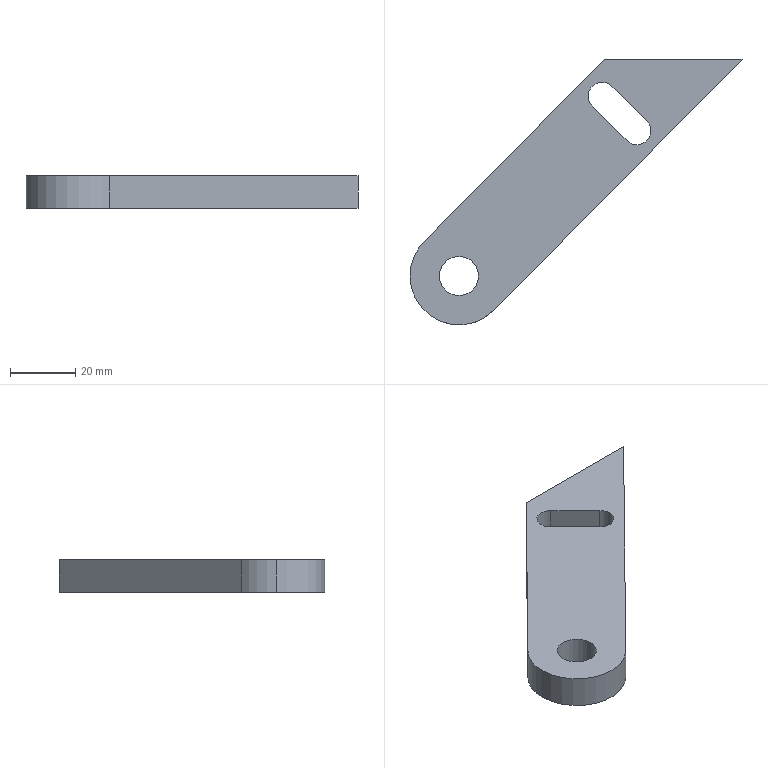Part | STEP file | Tensioning pulley fixing plate SGN-2-19 | 1 solid | 14 faces | box 101.738 x 81.439 x 10 mm | volume 28553 mm3 | cylinder 7 | plane 7 | commonest cylinder face diameters 8.6 x3 12 x2 30 x2
STEP:
#1=CARTESIAN_POINT('',(0.,0.,0.));
#2=DIRECTION('',(0.,0.,1.));
#3=DIRECTION('',(1.,0.,0.));
#4=AXIS2_PLACEMENT_3D('',#1,#2,#3);
#5=CARTESIAN_POINT('',(12.996,-18.86,0.));
#6=VERTEX_POINT('',#5);
#7=CARTESIAN_POINT('',(12.996,-18.86,10.));
#8=VERTEX_POINT('',#7);
#9=CARTESIAN_POINT('',(12.996,-18.86,0.));
#10=DIRECTION('',(0.,0.,1.));
#11=VECTOR('',#10,1.);
#12=LINE('',#9,#11);
#13=CARTESIAN_POINT('',(9.973,-21.919,0.));
#14=DIRECTION('',(0.,0.,1.));
#15=DIRECTION('',(1.,0.,0.));
#16=AXIS2_PLACEMENT_3D('',#13,#14,#15);
#17=CYLINDRICAL_SURFACE('',#16,4.3);
#18=CARTESIAN_POINT('',(0.7914,0.));
#19=DIRECTION('',(0.,1.));
#20=VECTOR('',#19,1.);
#21=LINE('',#18,#20);
#22=(GEOMETRIC_REPRESENTATION_CONTEXT(2)PARAMETRIC_REPRESENTATION_CONTEXT()REPRESENTATION_CONTEXT('',''));
#23=DEFINITIONAL_REPRESENTATION('',(#21),#22);
#24=PCURVE('',#17,#23);
#25=CARTESIAN_POINT('',(2.326,-8.317,0.));
#26=DIRECTION('',(0.7029,0.7113,0.));
#27=DIRECTION('',(-0.7113,0.7029,0.));
#28=AXIS2_PLACEMENT_3D('',#25,#26,#27);
#29=PLANE('',#28);
#30=CARTESIAN_POINT('',(-15.,0.));
#31=DIRECTION('',(0.,1.));
#32=VECTOR('',#31,1.);
#33=LINE('',#30,#32);
#34=(GEOMETRIC_REPRESENTATION_CONTEXT(2)PARAMETRIC_REPRESENTATION_CONTEXT()REPRESENTATION_CONTEXT('',''));
#35=DEFINITIONAL_REPRESENTATION('',(#33),#34);
#36=PCURVE('',#29,#35);
#37=SURFACE_CURVE('',#12,(#24,#36),.PCURVE_S1.);
#38=EDGE_CURVE('',#6,#8,#37,.T.);
#39=ORIENTED_EDGE('',*,*,#38,.T.);
#40=CARTESIAN_POINT('',(14.273,-21.919,10.));
#41=VERTEX_POINT('',#40);
#42=CARTESIAN_POINT('',(9.973,-21.919,10.));
#43=DIRECTION('',(0.,0.,1.));
#44=DIRECTION('',(1.,0.,0.));
#45=AXIS2_PLACEMENT_3D('',#42,#43,#44);
#46=CIRCLE('',#45,4.3);
#47=CARTESIAN_POINT('',(0.,10.));
#48=DIRECTION('',(1.,0.));
#49=VECTOR('',#48,1.);
#50=LINE('',#47,#49);
#51=(GEOMETRIC_REPRESENTATION_CONTEXT(2)PARAMETRIC_REPRESENTATION_CONTEXT()REPRESENTATION_CONTEXT('',''));
#52=DEFINITIONAL_REPRESENTATION('',(#50),#51);
#53=PCURVE('',#17,#52);
#54=CARTESIAN_POINT('',(-44.563,-66.439,10.));
#55=DIRECTION('',(0.,0.,1.));
#56=DIRECTION('',(1.,0.,0.));
#57=AXIS2_PLACEMENT_3D('',#54,#55,#56);
#58=PLANE('',#57);
#59=CARTESIAN_POINT('',(54.536,44.521));
#60=DIRECTION('',(1.,0.));
#61=AXIS2_PLACEMENT_2D('',#59,#60);
#62=CIRCLE('',#61,4.3);
#63=(GEOMETRIC_REPRESENTATION_CONTEXT(2)PARAMETRIC_REPRESENTATION_CONTEXT()REPRESENTATION_CONTEXT('',''));
#64=DEFINITIONAL_REPRESENTATION('',(#62),#63);
#65=PCURVE('',#58,#64);
#66=SURFACE_CURVE('',#46,(#53,#65),.PCURVE_S1.);
#67=EDGE_CURVE('',#41,#8,#66,.T.);
#68=ORIENTED_EDGE('',*,*,#67,.F.);
#69=CARTESIAN_POINT('',(14.273,-21.919,0.));
#70=VERTEX_POINT('',#69);
#71=CARTESIAN_POINT('',(14.273,-21.919,0.));
#72=DIRECTION('',(0.,0.,1.));
#73=VECTOR('',#72,1.);
#74=LINE('',#71,#73);
#75=CARTESIAN_POINT('',(0.,0.));
#76=DIRECTION('',(0.,1.));
#77=VECTOR('',#76,1.);
#78=LINE('',#75,#77);
#79=(GEOMETRIC_REPRESENTATION_CONTEXT(2)PARAMETRIC_REPRESENTATION_CONTEXT()REPRESENTATION_CONTEXT('',''));
#80=DEFINITIONAL_REPRESENTATION('',(#78),#79);
#81=PCURVE('',#17,#80);
#82=CARTESIAN_POINT('',(9.973,-21.919,0.));
#83=DIRECTION('',(0.,0.,1.));
#84=DIRECTION('',(1.,0.,0.));
#85=AXIS2_PLACEMENT_3D('',#82,#83,#84);
#86=CYLINDRICAL_SURFACE('',#85,4.3);
#87=CARTESIAN_POINT('',(6.283,0.));
#88=DIRECTION('',(0.,1.));
#89=VECTOR('',#88,1.);
#90=LINE('',#87,#89);
#91=(GEOMETRIC_REPRESENTATION_CONTEXT(2)PARAMETRIC_REPRESENTATION_CONTEXT()REPRESENTATION_CONTEXT('',''));
#92=DEFINITIONAL_REPRESENTATION('',(#90),#91);
#93=PCURVE('',#86,#92);
#94=SURFACE_CURVE('',#74,(#81,#93),.PCURVE_S1.);
#95=EDGE_CURVE('',#70,#41,#94,.T.);
#96=ORIENTED_EDGE('',*,*,#95,.F.);
#97=CARTESIAN_POINT('',(9.973,-21.919,0.));
#98=DIRECTION('',(0.,0.,1.));
#99=DIRECTION('',(1.,0.,0.));
#100=AXIS2_PLACEMENT_3D('',#97,#98,#99);
#101=CIRCLE('',#100,4.3);
#102=CARTESIAN_POINT('',(0.,0.));
#103=DIRECTION('',(1.,0.));
#104=VECTOR('',#103,1.);
#105=LINE('',#102,#104);
#106=(GEOMETRIC_REPRESENTATION_CONTEXT(2)PARAMETRIC_REPRESENTATION_CONTEXT()REPRESENTATION_CONTEXT('',''));
#107=DEFINITIONAL_REPRESENTATION('',(#105),#106);
#108=PCURVE('',#17,#107);
#109=CARTESIAN_POINT('',(-44.563,-66.439,0.));
#110=DIRECTION('',(0.,0.,1.));
#111=DIRECTION('',(1.,0.,0.));
#112=AXIS2_PLACEMENT_3D('',#109,#110,#111);
#113=PLANE('',#112);
#114=CARTESIAN_POINT('',(54.536,44.521));
#115=DIRECTION('',(1.,0.));
#116=AXIS2_PLACEMENT_2D('',#114,#115);
#117=CIRCLE('',#116,4.3);
#118=(GEOMETRIC_REPRESENTATION_CONTEXT(2)PARAMETRIC_REPRESENTATION_CONTEXT()REPRESENTATION_CONTEXT('',''));
#119=DEFINITIONAL_REPRESENTATION('',(#117),#118);
#120=PCURVE('',#113,#119);
#121=SURFACE_CURVE('',#101,(#108,#120),.PCURVE_S1.);
#122=EDGE_CURVE('',#70,#6,#121,.T.);
#123=ORIENTED_EDGE('',*,*,#122,.T.);
#124=EDGE_LOOP('',(#39,#68,#96,#123));
#125=FACE_BOUND('',#124,.F.);
#126=ADVANCED_FACE('',(#125),#17,.F.);
#127=CARTESIAN_POINT('',(-38.563,-66.439,0.));
#128=VERTEX_POINT('',#127);
#129=CARTESIAN_POINT('',(-38.563,-66.439,10.));
#130=VERTEX_POINT('',#129);
#131=CARTESIAN_POINT('',(-38.563,-66.439,10.));
#132=DIRECTION('',(0.,0.,1.));
#133=VECTOR('',#132,1.);
#134=LINE('',#131,#133);
#135=CARTESIAN_POINT('',(-44.563,-66.439,10.));
#136=DIRECTION('',(0.,0.,1.));
#137=DIRECTION('',(1.,0.,0.));
#138=AXIS2_PLACEMENT_3D('',#135,#136,#137);
#139=CYLINDRICAL_SURFACE('',#138,6.);
#140=CARTESIAN_POINT('',(6.283,0.));
#141=DIRECTION('',(0.,1.));
#142=VECTOR('',#141,1.);
#143=LINE('',#140,#142);
#144=(GEOMETRIC_REPRESENTATION_CONTEXT(2)PARAMETRIC_REPRESENTATION_CONTEXT()REPRESENTATION_CONTEXT('',''));
#145=DEFINITIONAL_REPRESENTATION('',(#143),#144);
#146=PCURVE('',#139,#145);
#147=CARTESIAN_POINT('',(-44.563,-66.439,10.));
#148=DIRECTION('',(0.,0.,1.));
#149=DIRECTION('',(1.,0.,0.));
#150=AXIS2_PLACEMENT_3D('',#147,#148,#149);
#151=CYLINDRICAL_SURFACE('',#150,6.);
#152=CARTESIAN_POINT('',(0.,0.));
#153=DIRECTION('',(0.,1.));
#154=VECTOR('',#153,1.);
#155=LINE('',#152,#154);
#156=(GEOMETRIC_REPRESENTATION_CONTEXT(2)PARAMETRIC_REPRESENTATION_CONTEXT()REPRESENTATION_CONTEXT('',''));
#157=DEFINITIONAL_REPRESENTATION('',(#155),#156);
#158=PCURVE('',#151,#157);
#159=SURFACE_CURVE('',#134,(#146,#158),.PCURVE_S1.);
#160=EDGE_CURVE('',#128,#130,#159,.T.);
#161=ORIENTED_EDGE('',*,*,#160,.T.);
#162=CARTESIAN_POINT('',(-50.563,-66.439,10.));
#163=VERTEX_POINT('',#162);
#164=CARTESIAN_POINT('',(-44.563,-66.439,10.));
#165=DIRECTION('',(0.,0.,1.));
#166=DIRECTION('',(1.,0.,0.));
#167=AXIS2_PLACEMENT_3D('',#164,#165,#166);
#168=CIRCLE('',#167,6.);
#169=CARTESIAN_POINT('',(0.,0.));
#170=DIRECTION('',(1.,0.));
#171=VECTOR('',#170,1.);
#172=LINE('',#169,#171);
#173=(GEOMETRIC_REPRESENTATION_CONTEXT(2)PARAMETRIC_REPRESENTATION_CONTEXT()REPRESENTATION_CONTEXT('',''));
#174=DEFINITIONAL_REPRESENTATION('',(#172),#173);
#175=PCURVE('',#139,#174);
#176=CARTESIAN_POINT('',(0.,0.));
#177=DIRECTION('',(1.,0.));
#178=AXIS2_PLACEMENT_2D('',#176,#177);
#179=CIRCLE('',#178,6.);
#180=(GEOMETRIC_REPRESENTATION_CONTEXT(2)PARAMETRIC_REPRESENTATION_CONTEXT()REPRESENTATION_CONTEXT('',''));
#181=DEFINITIONAL_REPRESENTATION('',(#179),#180);
#182=PCURVE('',#58,#181);
#183=SURFACE_CURVE('',#168,(#175,#182),.PCURVE_S1.);
#184=EDGE_CURVE('',#163,#130,#183,.T.);
#185=ORIENTED_EDGE('',*,*,#184,.F.);
#186=CARTESIAN_POINT('',(-50.563,-66.439,0.));
#187=VERTEX_POINT('',#186);
#188=CARTESIAN_POINT('',(-50.563,-66.439,10.));
#189=DIRECTION('',(0.,0.,1.));
#190=VECTOR('',#189,1.);
#191=LINE('',#188,#190);
#192=CARTESIAN_POINT('',(3.142,0.));
#193=DIRECTION('',(0.,1.));
#194=VECTOR('',#193,1.);
#195=LINE('',#192,#194);
#196=(GEOMETRIC_REPRESENTATION_CONTEXT(2)PARAMETRIC_REPRESENTATION_CONTEXT()REPRESENTATION_CONTEXT('',''));
#197=DEFINITIONAL_REPRESENTATION('',(#195),#196);
#198=PCURVE('',#139,#197);
#199=CARTESIAN_POINT('',(3.142,0.));
#200=DIRECTION('',(0.,1.));
#201=VECTOR('',#200,1.);
#202=LINE('',#199,#201);
#203=(GEOMETRIC_REPRESENTATION_CONTEXT(2)PARAMETRIC_REPRESENTATION_CONTEXT()REPRESENTATION_CONTEXT('',''));
#204=DEFINITIONAL_REPRESENTATION('',(#202),#203);
#205=PCURVE('',#151,#204);
#206=SURFACE_CURVE('',#191,(#198,#205),.PCURVE_S1.);
#207=EDGE_CURVE('',#187,#163,#206,.T.);
#208=ORIENTED_EDGE('',*,*,#207,.F.);
#209=CARTESIAN_POINT('',(-44.563,-66.439,0.));
#210=DIRECTION('',(0.,0.,1.));
#211=DIRECTION('',(1.,0.,0.));
#212=AXIS2_PLACEMENT_3D('',#209,#210,#211);
#213=CIRCLE('',#212,6.);
#214=CARTESIAN_POINT('',(0.,-10.));
#215=DIRECTION('',(1.,0.));
#216=VECTOR('',#215,1.);
#217=LINE('',#214,#216);
#218=(GEOMETRIC_REPRESENTATION_CONTEXT(2)PARAMETRIC_REPRESENTATION_CONTEXT()REPRESENTATION_CONTEXT('',''));
#219=DEFINITIONAL_REPRESENTATION('',(#217),#218);
#220=PCURVE('',#139,#219);
#221=CARTESIAN_POINT('',(0.,0.));
#222=DIRECTION('',(1.,0.));
#223=AXIS2_PLACEMENT_2D('',#221,#222);
#224=CIRCLE('',#223,6.);
#225=(GEOMETRIC_REPRESENTATION_CONTEXT(2)PARAMETRIC_REPRESENTATION_CONTEXT()REPRESENTATION_CONTEXT('',''));
#226=DEFINITIONAL_REPRESENTATION('',(#224),#225);
#227=PCURVE('',#113,#226);
#228=SURFACE_CURVE('',#213,(#220,#227),.PCURVE_S1.);
#229=EDGE_CURVE('',#187,#128,#228,.T.);
#230=ORIENTED_EDGE('',*,*,#229,.T.);
#231=EDGE_LOOP('',(#161,#185,#208,#230));
#232=FACE_BOUND('',#231,.F.);
#233=ADVANCED_FACE('',(#232),#139,.F.);
#234=CARTESIAN_POINT('',(-59.563,-66.439,10.));
#235=VERTEX_POINT('',#234);
#236=CARTESIAN_POINT('',(-33.893,-76.982,10.));
#237=VERTEX_POINT('',#236);
#238=CARTESIAN_POINT('',(-44.563,-66.439,10.));
#239=DIRECTION('',(0.,0.,1.));
#240=DIRECTION('',(1.,0.,0.));
#241=AXIS2_PLACEMENT_3D('',#238,#239,#240);
#242=CIRCLE('',#241,15.);
#243=CARTESIAN_POINT('',(-44.563,-66.439,10.));
#244=DIRECTION('',(0.,0.,-1.));
#245=DIRECTION('',(-1.,0.,0.));
#246=AXIS2_PLACEMENT_3D('',#243,#244,#245);
#247=CYLINDRICAL_SURFACE('',#246,15.);
#248=CARTESIAN_POINT('',(9.425,0.));
#249=DIRECTION('',(-1.,0.));
#250=VECTOR('',#249,1.);
#251=LINE('',#248,#250);
#252=(GEOMETRIC_REPRESENTATION_CONTEXT(2)PARAMETRIC_REPRESENTATION_CONTEXT()REPRESENTATION_CONTEXT('',''));
#253=DEFINITIONAL_REPRESENTATION('',(#251),#252);
#254=PCURVE('',#247,#253);
#255=CARTESIAN_POINT('',(0.,0.));
#256=DIRECTION('',(1.,0.));
#257=AXIS2_PLACEMENT_2D('',#255,#256);
#258=CIRCLE('',#257,15.);
#259=(GEOMETRIC_REPRESENTATION_CONTEXT(2)PARAMETRIC_REPRESENTATION_CONTEXT()REPRESENTATION_CONTEXT('',''));
#260=DEFINITIONAL_REPRESENTATION('',(#258),#259);
#261=PCURVE('',#58,#260);
#262=SURFACE_CURVE('',#242,(#254,#261),.PCURVE_S1.);
#263=EDGE_CURVE('',#235,#237,#262,.T.);
#264=ORIENTED_EDGE('',*,*,#263,.F.);
#265=CARTESIAN_POINT('',(-59.563,-66.439,0.));
#266=VERTEX_POINT('',#265);
#267=CARTESIAN_POINT('',(-59.563,-66.439,10.));
#268=DIRECTION('',(0.,0.,-1.));
#269=VECTOR('',#268,1.);
#270=LINE('',#267,#269);
#271=CARTESIAN_POINT('',(6.283,0.));
#272=DIRECTION('',(0.,1.));
#273=VECTOR('',#272,1.);
#274=LINE('',#271,#273);
#275=(GEOMETRIC_REPRESENTATION_CONTEXT(2)PARAMETRIC_REPRESENTATION_CONTEXT()REPRESENTATION_CONTEXT('',''));
#276=DEFINITIONAL_REPRESENTATION('',(#274),#275);
#277=PCURVE('',#247,#276);
#278=CARTESIAN_POINT('',(-44.563,-66.439,10.));
#279=DIRECTION('',(0.,0.,-1.));
#280=DIRECTION('',(-1.,0.,0.));
#281=AXIS2_PLACEMENT_3D('',#278,#279,#280);
#282=CYLINDRICAL_SURFACE('',#281,15.);
#283=CARTESIAN_POINT('',(0.,0.));
#284=DIRECTION('',(0.,1.));
#285=VECTOR('',#284,1.);
#286=LINE('',#283,#285);
#287=(GEOMETRIC_REPRESENTATION_CONTEXT(2)PARAMETRIC_REPRESENTATION_CONTEXT()REPRESENTATION_CONTEXT('',''));
#288=DEFINITIONAL_REPRESENTATION('',(#286),#287);
#289=PCURVE('',#282,#288);
#290=SURFACE_CURVE('',#270,(#277,#289),.PCURVE_S1.);
#291=EDGE_CURVE('',#235,#266,#290,.T.);
#292=ORIENTED_EDGE('',*,*,#291,.T.);
#293=CARTESIAN_POINT('',(-33.893,-76.982,0.));
#294=VERTEX_POINT('',#293);
#295=CARTESIAN_POINT('',(-44.563,-66.439,0.));
#296=DIRECTION('',(0.,0.,1.));
#297=DIRECTION('',(1.,0.,0.));
#298=AXIS2_PLACEMENT_3D('',#295,#296,#297);
#299=CIRCLE('',#298,15.);
#300=CARTESIAN_POINT('',(9.425,10.));
#301=DIRECTION('',(-1.,0.));
#302=VECTOR('',#301,1.);
#303=LINE('',#300,#302);
#304=(GEOMETRIC_REPRESENTATION_CONTEXT(2)PARAMETRIC_REPRESENTATION_CONTEXT()REPRESENTATION_CONTEXT('',''));
#305=DEFINITIONAL_REPRESENTATION('',(#303),#304);
#306=PCURVE('',#247,#305);
#307=CARTESIAN_POINT('',(0.,0.));
#308=DIRECTION('',(1.,0.));
#309=AXIS2_PLACEMENT_2D('',#307,#308);
#310=CIRCLE('',#309,15.);
#311=(GEOMETRIC_REPRESENTATION_CONTEXT(2)PARAMETRIC_REPRESENTATION_CONTEXT()REPRESENTATION_CONTEXT('',''));
#312=DEFINITIONAL_REPRESENTATION('',(#310),#311);
#313=PCURVE('',#113,#312);
#314=SURFACE_CURVE('',#299,(#306,#313),.PCURVE_S1.);
#315=EDGE_CURVE('',#266,#294,#314,.T.);
#316=ORIENTED_EDGE('',*,*,#315,.T.);
#317=CARTESIAN_POINT('',(-33.893,-76.982,10.));
#318=DIRECTION('',(0.,0.,-1.));
#319=VECTOR('',#318,1.);
#320=LINE('',#317,#319);
#321=CARTESIAN_POINT('',(3.921,0.));
#322=DIRECTION('',(0.,1.));
#323=VECTOR('',#322,1.);
#324=LINE('',#321,#323);
#325=(GEOMETRIC_REPRESENTATION_CONTEXT(2)PARAMETRIC_REPRESENTATION_CONTEXT()REPRESENTATION_CONTEXT('',''));
#326=DEFINITIONAL_REPRESENTATION('',(#324),#325);
#327=PCURVE('',#247,#326);
#328=CARTESIAN_POINT('',(42.175,0.,10.));
#329=DIRECTION('',(-0.7113,0.7029,0.));
#330=DIRECTION('',(-0.7029,-0.7113,0.));
#331=AXIS2_PLACEMENT_3D('',#328,#329,#330);
#332=PLANE('',#331);
#333=CARTESIAN_POINT('',(108.225,0.));
#334=DIRECTION('',(0.,-1.));
#335=VECTOR('',#334,1.);
#336=LINE('',#333,#335);
#337=(GEOMETRIC_REPRESENTATION_CONTEXT(2)PARAMETRIC_REPRESENTATION_CONTEXT()REPRESENTATION_CONTEXT('',''));
#338=DEFINITIONAL_REPRESENTATION('',(#336),#337);
#339=PCURVE('',#332,#338);
#340=SURFACE_CURVE('',#320,(#327,#339),.PCURVE_S1.);
#341=EDGE_CURVE('',#237,#294,#340,.T.);
#342=ORIENTED_EDGE('',*,*,#341,.F.);
#343=EDGE_LOOP('',(#264,#292,#316,#342));
#344=FACE_BOUND('',#343,.T.);
#345=ADVANCED_FACE('',(#344),#247,.T.);
#346=CARTESIAN_POINT('',(0.,0.,0.));
#347=VERTEX_POINT('',#346);
#348=CARTESIAN_POINT('',(-55.232,-55.896,0.));
#349=VERTEX_POINT('',#348);
#350=CARTESIAN_POINT('',(0.,0.,0.));
#351=DIRECTION('',(-0.7029,-0.7113,0.));
#352=VECTOR('',#351,1.);
#353=LINE('',#350,#352);
#354=CARTESIAN_POINT('',(0.,0.,10.));
#355=DIRECTION('',(0.7113,-0.7029,0.));
#356=DIRECTION('',(0.7029,0.7113,0.));
#357=AXIS2_PLACEMENT_3D('',#354,#355,#356);
#358=PLANE('',#357);
#359=CARTESIAN_POINT('',(0.,-10.));
#360=DIRECTION('',(-1.,0.));
#361=VECTOR('',#360,1.);
#362=LINE('',#359,#361);
#363=(GEOMETRIC_REPRESENTATION_CONTEXT(2)PARAMETRIC_REPRESENTATION_CONTEXT()REPRESENTATION_CONTEXT('',''));
#364=DEFINITIONAL_REPRESENTATION('',(#362),#363);
#365=PCURVE('',#358,#364);
#366=CARTESIAN_POINT('',(44.563,66.439));
#367=DIRECTION('',(-0.7029,-0.7113));
#368=VECTOR('',#367,1.);
#369=LINE('',#366,#368);
#370=(GEOMETRIC_REPRESENTATION_CONTEXT(2)PARAMETRIC_REPRESENTATION_CONTEXT()REPRESENTATION_CONTEXT('',''));
#371=DEFINITIONAL_REPRESENTATION('',(#369),#370);
#372=PCURVE('',#113,#371);
#373=SURFACE_CURVE('',#353,(#365,#372),.PCURVE_S1.);
#374=EDGE_CURVE('',#347,#349,#373,.T.);
#375=ORIENTED_EDGE('',*,*,#374,.T.);
#376=CARTESIAN_POINT('',(-55.232,-55.896,10.));
#377=VERTEX_POINT('',#376);
#378=CARTESIAN_POINT('',(-55.232,-55.896,10.));
#379=DIRECTION('',(0.,0.,-1.));
#380=VECTOR('',#379,1.);
#381=LINE('',#378,#380);
#382=CARTESIAN_POINT('',(-78.581,0.));
#383=DIRECTION('',(0.,-1.));
#384=VECTOR('',#383,1.);
#385=LINE('',#382,#384);
#386=(GEOMETRIC_REPRESENTATION_CONTEXT(2)PARAMETRIC_REPRESENTATION_CONTEXT()REPRESENTATION_CONTEXT('',''));
#387=DEFINITIONAL_REPRESENTATION('',(#385),#386);
#388=PCURVE('',#358,#387);
#389=CARTESIAN_POINT('',(0.7794,0.));
#390=DIRECTION('',(0.,1.));
#391=VECTOR('',#390,1.);
#392=LINE('',#389,#391);
#393=(GEOMETRIC_REPRESENTATION_CONTEXT(2)PARAMETRIC_REPRESENTATION_CONTEXT()REPRESENTATION_CONTEXT('',''));
#394=DEFINITIONAL_REPRESENTATION('',(#392),#393);
#395=PCURVE('',#282,#394);
#396=SURFACE_CURVE('',#381,(#388,#395),.PCURVE_S1.);
#397=EDGE_CURVE('',#377,#349,#396,.T.);
#398=ORIENTED_EDGE('',*,*,#397,.F.);
#399=CARTESIAN_POINT('',(0.,0.,10.));
#400=VERTEX_POINT('',#399);
#401=CARTESIAN_POINT('',(0.,0.,10.));
#402=DIRECTION('',(-0.7029,-0.7113,0.));
#403=VECTOR('',#402,1.);
#404=LINE('',#401,#403);
#405=CARTESIAN_POINT('',(0.,0.));
#406=DIRECTION('',(-1.,0.));
#407=VECTOR('',#406,1.);
#408=LINE('',#405,#407);
#409=(GEOMETRIC_REPRESENTATION_CONTEXT(2)PARAMETRIC_REPRESENTATION_CONTEXT()REPRESENTATION_CONTEXT('',''));
#410=DEFINITIONAL_REPRESENTATION('',(#408),#409);
#411=PCURVE('',#358,#410);
#412=CARTESIAN_POINT('',(44.563,66.439));
#413=DIRECTION('',(-0.7029,-0.7113));
#414=VECTOR('',#413,1.);
#415=LINE('',#412,#414);
#416=(GEOMETRIC_REPRESENTATION_CONTEXT(2)PARAMETRIC_REPRESENTATION_CONTEXT()REPRESENTATION_CONTEXT('',''));
#417=DEFINITIONAL_REPRESENTATION('',(#415),#416);
#418=PCURVE('',#58,#417);
#419=SURFACE_CURVE('',#404,(#411,#418),.PCURVE_S1.);
#420=EDGE_CURVE('',#400,#377,#419,.T.);
#421=ORIENTED_EDGE('',*,*,#420,.F.);
#422=CARTESIAN_POINT('',(0.,0.,10.));
#423=DIRECTION('',(0.,0.,-1.));
#424=VECTOR('',#423,1.);
#425=LINE('',#422,#424);
#426=CARTESIAN_POINT('',(0.,0.));
#427=DIRECTION('',(0.,-1.));
#428=VECTOR('',#427,1.);
#429=LINE('',#426,#428);
#430=(GEOMETRIC_REPRESENTATION_CONTEXT(2)PARAMETRIC_REPRESENTATION_CONTEXT()REPRESENTATION_CONTEXT('',''));
#431=DEFINITIONAL_REPRESENTATION('',(#429),#430);
#432=PCURVE('',#358,#431);
#433=CARTESIAN_POINT('',(0.,0.,10.));
#434=DIRECTION('',(0.,-1.,0.));
#435=DIRECTION('',(0.,0.,-1.));
#436=AXIS2_PLACEMENT_3D('',#433,#434,#435);
#437=PLANE('',#436);
#438=CARTESIAN_POINT('',(0.,0.));
#439=DIRECTION('',(1.,0.));
#440=VECTOR('',#439,1.);
#441=LINE('',#438,#440);
#442=(GEOMETRIC_REPRESENTATION_CONTEXT(2)PARAMETRIC_REPRESENTATION_CONTEXT()REPRESENTATION_CONTEXT('',''));
#443=DEFINITIONAL_REPRESENTATION('',(#441),#442);
#444=PCURVE('',#437,#443);
#445=SURFACE_CURVE('',#425,(#432,#444),.PCURVE_S1.);
#446=EDGE_CURVE('',#400,#347,#445,.T.);
#447=ORIENTED_EDGE('',*,*,#446,.T.);
#448=EDGE_LOOP('',(#375,#398,#421,#447));
#449=FACE_BOUND('',#448,.T.);
#450=ADVANCED_FACE('',(#449),#358,.F.);
#451=ORIENTED_EDGE('',*,*,#291,.F.);
#452=CARTESIAN_POINT('',(-44.563,-66.439,10.));
#453=DIRECTION('',(0.,0.,1.));
#454=DIRECTION('',(1.,0.,0.));
#455=AXIS2_PLACEMENT_3D('',#452,#453,#454);
#456=CIRCLE('',#455,15.);
#457=CARTESIAN_POINT('',(3.142,0.));
#458=DIRECTION('',(-1.,0.));
#459=VECTOR('',#458,1.);
#460=LINE('',#457,#459);
#461=(GEOMETRIC_REPRESENTATION_CONTEXT(2)PARAMETRIC_REPRESENTATION_CONTEXT()REPRESENTATION_CONTEXT('',''));
#462=DEFINITIONAL_REPRESENTATION('',(#460),#461);
#463=PCURVE('',#282,#462);
#464=CARTESIAN_POINT('',(0.,0.));
#465=DIRECTION('',(1.,0.));
#466=AXIS2_PLACEMENT_2D('',#464,#465);
#467=CIRCLE('',#466,15.);
#468=(GEOMETRIC_REPRESENTATION_CONTEXT(2)PARAMETRIC_REPRESENTATION_CONTEXT()REPRESENTATION_CONTEXT('',''));
#469=DEFINITIONAL_REPRESENTATION('',(#467),#468);
#470=PCURVE('',#58,#469);
#471=SURFACE_CURVE('',#456,(#463,#470),.PCURVE_S1.);
#472=EDGE_CURVE('',#377,#235,#471,.T.);
#473=ORIENTED_EDGE('',*,*,#472,.F.);
#474=ORIENTED_EDGE('',*,*,#397,.T.);
#475=CARTESIAN_POINT('',(-44.563,-66.439,0.));
#476=DIRECTION('',(0.,0.,1.));
#477=DIRECTION('',(1.,0.,0.));
#478=AXIS2_PLACEMENT_3D('',#475,#476,#477);
#479=CIRCLE('',#478,15.);
#480=CARTESIAN_POINT('',(3.142,10.));
#481=DIRECTION('',(-1.,0.));
#482=VECTOR('',#481,1.);
#483=LINE('',#480,#482);
#484=(GEOMETRIC_REPRESENTATION_CONTEXT(2)PARAMETRIC_REPRESENTATION_CONTEXT()REPRESENTATION_CONTEXT('',''));
#485=DEFINITIONAL_REPRESENTATION('',(#483),#484);
#486=PCURVE('',#282,#485);
#487=CARTESIAN_POINT('',(0.,0.));
#488=DIRECTION('',(1.,0.));
#489=AXIS2_PLACEMENT_2D('',#487,#488);
#490=CIRCLE('',#489,15.);
#491=(GEOMETRIC_REPRESENTATION_CONTEXT(2)PARAMETRIC_REPRESENTATION_CONTEXT()REPRESENTATION_CONTEXT('',''));
#492=DEFINITIONAL_REPRESENTATION('',(#490),#491);
#493=PCURVE('',#113,#492);
#494=SURFACE_CURVE('',#479,(#486,#493),.PCURVE_S1.);
#495=EDGE_CURVE('',#349,#266,#494,.T.);
#496=ORIENTED_EDGE('',*,*,#495,.T.);
#497=EDGE_LOOP('',(#451,#473,#474,#496));
#498=FACE_BOUND('',#497,.T.);
#499=ADVANCED_FACE('',(#498),#282,.T.);
#500=CARTESIAN_POINT('',(42.175,0.,0.));
#501=VERTEX_POINT('',#500);
#502=CARTESIAN_POINT('',(42.175,0.,0.));
#503=DIRECTION('',(0.7029,0.7113,0.));
#504=VECTOR('',#503,1.);
#505=LINE('',#502,#504);
#506=CARTESIAN_POINT('',(0.,-10.));
#507=DIRECTION('',(-1.,0.));
#508=VECTOR('',#507,1.);
#509=LINE('',#506,#508);
#510=(GEOMETRIC_REPRESENTATION_CONTEXT(2)PARAMETRIC_REPRESENTATION_CONTEXT()REPRESENTATION_CONTEXT('',''));
#511=DEFINITIONAL_REPRESENTATION('',(#509),#510);
#512=PCURVE('',#332,#511);
#513=CARTESIAN_POINT('',(86.738,66.439));
#514=DIRECTION('',(0.7029,0.7113));
#515=VECTOR('',#514,1.);
#516=LINE('',#513,#515);
#517=(GEOMETRIC_REPRESENTATION_CONTEXT(2)PARAMETRIC_REPRESENTATION_CONTEXT()REPRESENTATION_CONTEXT('',''));
#518=DEFINITIONAL_REPRESENTATION('',(#516),#517);
#519=PCURVE('',#113,#518);
#520=SURFACE_CURVE('',#505,(#512,#519),.PCURVE_S1.);
#521=EDGE_CURVE('',#294,#501,#520,.T.);
#522=ORIENTED_EDGE('',*,*,#521,.T.);
#523=CARTESIAN_POINT('',(42.175,0.,10.));
#524=VERTEX_POINT('',#523);
#525=CARTESIAN_POINT('',(42.175,0.,10.));
#526=DIRECTION('',(0.,0.,-1.));
#527=VECTOR('',#526,1.);
#528=LINE('',#525,#527);
#529=CARTESIAN_POINT('',(0.,0.));
#530=DIRECTION('',(0.,-1.));
#531=VECTOR('',#530,1.);
#532=LINE('',#529,#531);
#533=(GEOMETRIC_REPRESENTATION_CONTEXT(2)PARAMETRIC_REPRESENTATION_CONTEXT()REPRESENTATION_CONTEXT('',''));
#534=DEFINITIONAL_REPRESENTATION('',(#532),#533);
#535=PCURVE('',#332,#534);
#536=CARTESIAN_POINT('',(0.,42.175));
#537=DIRECTION('',(1.,0.));
#538=VECTOR('',#537,1.);
#539=LINE('',#536,#538);
#540=(GEOMETRIC_REPRESENTATION_CONTEXT(2)PARAMETRIC_REPRESENTATION_CONTEXT()REPRESENTATION_CONTEXT('',''));
#541=DEFINITIONAL_REPRESENTATION('',(#539),#540);
#542=PCURVE('',#437,#541);
#543=SURFACE_CURVE('',#528,(#535,#542),.PCURVE_S1.);
#544=EDGE_CURVE('',#524,#501,#543,.T.);
#545=ORIENTED_EDGE('',*,*,#544,.F.);
#546=CARTESIAN_POINT('',(42.175,0.,10.));
#547=DIRECTION('',(0.7029,0.7113,0.));
#548=VECTOR('',#547,1.);
#549=LINE('',#546,#548);
#550=CARTESIAN_POINT('',(0.,0.));
#551=DIRECTION('',(-1.,0.));
#552=VECTOR('',#551,1.);
#553=LINE('',#550,#552);
#554=(GEOMETRIC_REPRESENTATION_CONTEXT(2)PARAMETRIC_REPRESENTATION_CONTEXT()REPRESENTATION_CONTEXT('',''));
#555=DEFINITIONAL_REPRESENTATION('',(#553),#554);
#556=PCURVE('',#332,#555);
#557=CARTESIAN_POINT('',(86.738,66.439));
#558=DIRECTION('',(0.7029,0.7113));
#559=VECTOR('',#558,1.);
#560=LINE('',#557,#559);
#561=(GEOMETRIC_REPRESENTATION_CONTEXT(2)PARAMETRIC_REPRESENTATION_CONTEXT()REPRESENTATION_CONTEXT('',''));
#562=DEFINITIONAL_REPRESENTATION('',(#560),#561);
#563=PCURVE('',#58,#562);
#564=SURFACE_CURVE('',#549,(#556,#563),.PCURVE_S1.);
#565=EDGE_CURVE('',#237,#524,#564,.T.);
#566=ORIENTED_EDGE('',*,*,#565,.F.);
#567=ORIENTED_EDGE('',*,*,#341,.T.);
#568=EDGE_LOOP('',(#522,#545,#566,#567));
#569=FACE_BOUND('',#568,.T.);
#570=ADVANCED_FACE('',(#569),#332,.F.);
#571=CARTESIAN_POINT('',(0.,0.,0.));
#572=DIRECTION('',(-1.,0.,0.));
#573=VECTOR('',#572,1.);
#574=LINE('',#571,#573);
#575=CARTESIAN_POINT('',(10.,0.));
#576=DIRECTION('',(0.,-1.));
#577=VECTOR('',#576,1.);
#578=LINE('',#575,#577);
#579=(GEOMETRIC_REPRESENTATION_CONTEXT(2)PARAMETRIC_REPRESENTATION_CONTEXT()REPRESENTATION_CONTEXT('',''));
#580=DEFINITIONAL_REPRESENTATION('',(#578),#579);
#581=PCURVE('',#437,#580);
#582=CARTESIAN_POINT('',(44.563,66.439));
#583=DIRECTION('',(-1.,0.));
#584=VECTOR('',#583,1.);
#585=LINE('',#582,#584);
#586=(GEOMETRIC_REPRESENTATION_CONTEXT(2)PARAMETRIC_REPRESENTATION_CONTEXT()REPRESENTATION_CONTEXT('',''));
#587=DEFINITIONAL_REPRESENTATION('',(#585),#586);
#588=PCURVE('',#113,#587);
#589=SURFACE_CURVE('',#574,(#581,#588),.PCURVE_S1.);
#590=EDGE_CURVE('',#501,#347,#589,.T.);
#591=ORIENTED_EDGE('',*,*,#590,.T.);
#592=ORIENTED_EDGE('',*,*,#446,.F.);
#593=CARTESIAN_POINT('',(0.,0.,10.));
#594=DIRECTION('',(-1.,0.,0.));
#595=VECTOR('',#594,1.);
#596=LINE('',#593,#595);
#597=CARTESIAN_POINT('',(0.,0.));
#598=DIRECTION('',(0.,-1.));
#599=VECTOR('',#598,1.);
#600=LINE('',#597,#599);
#601=(GEOMETRIC_REPRESENTATION_CONTEXT(2)PARAMETRIC_REPRESENTATION_CONTEXT()REPRESENTATION_CONTEXT('',''));
#602=DEFINITIONAL_REPRESENTATION('',(#600),#601);
#603=PCURVE('',#437,#602);
#604=CARTESIAN_POINT('',(44.563,66.439));
#605=DIRECTION('',(-1.,0.));
#606=VECTOR('',#605,1.);
#607=LINE('',#604,#606);
#608=(GEOMETRIC_REPRESENTATION_CONTEXT(2)PARAMETRIC_REPRESENTATION_CONTEXT()REPRESENTATION_CONTEXT('',''));
#609=DEFINITIONAL_REPRESENTATION('',(#607),#608);
#610=PCURVE('',#58,#609);
#611=SURFACE_CURVE('',#596,(#603,#610),.PCURVE_S1.);
#612=EDGE_CURVE('',#524,#400,#611,.T.);
#613=ORIENTED_EDGE('',*,*,#612,.F.);
#614=ORIENTED_EDGE('',*,*,#544,.T.);
#615=EDGE_LOOP('',(#591,#592,#613,#614));
#616=FACE_BOUND('',#615,.T.);
#617=ADVANCED_FACE('',(#616),#437,.F.);
#618=CARTESIAN_POINT('',(2.326,-8.317,10.));
#619=VERTEX_POINT('',#618);
#620=CARTESIAN_POINT('',(-3.719,-14.434,10.));
#621=VERTEX_POINT('',#620);
#622=CARTESIAN_POINT('',(-0.6966,-11.375,10.));
#623=DIRECTION('',(0.,0.,1.));
#624=DIRECTION('',(1.,0.,0.));
#625=AXIS2_PLACEMENT_3D('',#622,#623,#624);
#626=CIRCLE('',#625,4.3);
#627=CARTESIAN_POINT('',(43.866,55.064));
#628=DIRECTION('',(1.,0.));
#629=AXIS2_PLACEMENT_2D('',#627,#628);
#630=CIRCLE('',#629,4.3);
#631=(GEOMETRIC_REPRESENTATION_CONTEXT(2)PARAMETRIC_REPRESENTATION_CONTEXT()REPRESENTATION_CONTEXT('',''));
#632=DEFINITIONAL_REPRESENTATION('',(#630),#631);
#633=PCURVE('',#58,#632);
#634=CARTESIAN_POINT('',(-0.6966,-11.375,0.));
#635=DIRECTION('',(0.,0.,1.));
#636=DIRECTION('',(1.,0.,0.));
#637=AXIS2_PLACEMENT_3D('',#634,#635,#636);
#638=CYLINDRICAL_SURFACE('',#637,4.3);
#639=CARTESIAN_POINT('',(0.,10.));
#640=DIRECTION('',(1.,0.));
#641=VECTOR('',#640,1.);
#642=LINE('',#639,#641);
#643=(GEOMETRIC_REPRESENTATION_CONTEXT(2)PARAMETRIC_REPRESENTATION_CONTEXT()REPRESENTATION_CONTEXT('',''));
#644=DEFINITIONAL_REPRESENTATION('',(#642),#643);
#645=PCURVE('',#638,#644);
#646=SURFACE_CURVE('',#626,(#633,#645),.PCURVE_S1.);
#647=EDGE_CURVE('',#619,#621,#646,.T.);
#648=ORIENTED_EDGE('',*,*,#647,.F.);
#649=CARTESIAN_POINT('',(2.326,-8.317,10.));
#650=DIRECTION('',(-0.7113,0.7029,0.));
#651=VECTOR('',#650,1.);
#652=LINE('',#649,#651);
#653=CARTESIAN_POINT('',(46.889,58.122));
#654=DIRECTION('',(-0.7113,0.7029));
#655=VECTOR('',#654,1.);
#656=LINE('',#653,#655);
#657=(GEOMETRIC_REPRESENTATION_CONTEXT(2)PARAMETRIC_REPRESENTATION_CONTEXT()REPRESENTATION_CONTEXT('',''));
#658=DEFINITIONAL_REPRESENTATION('',(#656),#657);
#659=PCURVE('',#58,#658);
#660=CARTESIAN_POINT('',(0.,10.));
#661=DIRECTION('',(1.,0.));
#662=VECTOR('',#661,1.);
#663=LINE('',#660,#662);
#664=(GEOMETRIC_REPRESENTATION_CONTEXT(2)PARAMETRIC_REPRESENTATION_CONTEXT()REPRESENTATION_CONTEXT('',''));
#665=DEFINITIONAL_REPRESENTATION('',(#663),#664);
#666=PCURVE('',#29,#665);
#667=SURFACE_CURVE('',#652,(#659,#666),.PCURVE_S1.);
#668=EDGE_CURVE('',#8,#619,#667,.T.);
#669=ORIENTED_EDGE('',*,*,#668,.F.);
#670=ORIENTED_EDGE('',*,*,#67,.F.);
#671=CARTESIAN_POINT('',(6.951,-24.977,10.));
#672=VERTEX_POINT('',#671);
#673=CARTESIAN_POINT('',(9.973,-21.919,10.));
#674=DIRECTION('',(0.,0.,1.));
#675=DIRECTION('',(1.,0.,0.));
#676=AXIS2_PLACEMENT_3D('',#673,#674,#675);
#677=CIRCLE('',#676,4.3);
#678=CARTESIAN_POINT('',(54.536,44.521));
#679=DIRECTION('',(1.,0.));
#680=AXIS2_PLACEMENT_2D('',#678,#679);
#681=CIRCLE('',#680,4.3);
#682=(GEOMETRIC_REPRESENTATION_CONTEXT(2)PARAMETRIC_REPRESENTATION_CONTEXT()REPRESENTATION_CONTEXT('',''));
#683=DEFINITIONAL_REPRESENTATION('',(#681),#682);
#684=PCURVE('',#58,#683);
#685=CARTESIAN_POINT('',(0.,10.));
#686=DIRECTION('',(1.,0.));
#687=VECTOR('',#686,1.);
#688=LINE('',#685,#687);
#689=(GEOMETRIC_REPRESENTATION_CONTEXT(2)PARAMETRIC_REPRESENTATION_CONTEXT()REPRESENTATION_CONTEXT('',''));
#690=DEFINITIONAL_REPRESENTATION('',(#688),#689);
#691=PCURVE('',#86,#690);
#692=SURFACE_CURVE('',#677,(#684,#691),.PCURVE_S1.);
#693=EDGE_CURVE('',#672,#41,#692,.T.);
#694=ORIENTED_EDGE('',*,*,#693,.F.);
#695=CARTESIAN_POINT('',(-3.719,-14.434,10.));
#696=DIRECTION('',(0.7113,-0.7029,0.));
#697=VECTOR('',#696,1.);
#698=LINE('',#695,#697);
#699=CARTESIAN_POINT('',(40.844,52.005));
#700=DIRECTION('',(0.7113,-0.7029));
#701=VECTOR('',#700,1.);
#702=LINE('',#699,#701);
#703=(GEOMETRIC_REPRESENTATION_CONTEXT(2)PARAMETRIC_REPRESENTATION_CONTEXT()REPRESENTATION_CONTEXT('',''));
#704=DEFINITIONAL_REPRESENTATION('',(#702),#703);
#705=PCURVE('',#58,#704);
#706=CARTESIAN_POINT('',(-3.719,-14.434,0.));
#707=DIRECTION('',(-0.7029,-0.7113,0.));
#708=DIRECTION('',(0.7113,-0.7029,0.));
#709=AXIS2_PLACEMENT_3D('',#706,#707,#708);
#710=PLANE('',#709);
#711=CARTESIAN_POINT('',(0.,10.));
#712=DIRECTION('',(1.,0.));
#713=VECTOR('',#712,1.);
#714=LINE('',#711,#713);
#715=(GEOMETRIC_REPRESENTATION_CONTEXT(2)PARAMETRIC_REPRESENTATION_CONTEXT()REPRESENTATION_CONTEXT('',''));
#716=DEFINITIONAL_REPRESENTATION('',(#714),#715);
#717=PCURVE('',#710,#716);
#718=SURFACE_CURVE('',#698,(#705,#717),.PCURVE_S1.);
#719=EDGE_CURVE('',#621,#672,#718,.T.);
#720=ORIENTED_EDGE('',*,*,#719,.F.);
#721=EDGE_LOOP('',(#648,#669,#670,#694,#720));
#722=FACE_BOUND('',#721,.T.);
#723=CARTESIAN_POINT('',(-44.563,-66.439,10.));
#724=DIRECTION('',(0.,0.,1.));
#725=DIRECTION('',(1.,0.,0.));
#726=AXIS2_PLACEMENT_3D('',#723,#724,#725);
#727=CIRCLE('',#726,6.);
#728=CARTESIAN_POINT('',(0.,0.));
#729=DIRECTION('',(1.,0.));
#730=AXIS2_PLACEMENT_2D('',#728,#729);
#731=CIRCLE('',#730,6.);
#732=(GEOMETRIC_REPRESENTATION_CONTEXT(2)PARAMETRIC_REPRESENTATION_CONTEXT()REPRESENTATION_CONTEXT('',''));
#733=DEFINITIONAL_REPRESENTATION('',(#731),#732);
#734=PCURVE('',#58,#733);
#735=CARTESIAN_POINT('',(0.,0.));
#736=DIRECTION('',(1.,0.));
#737=VECTOR('',#736,1.);
#738=LINE('',#735,#737);
#739=(GEOMETRIC_REPRESENTATION_CONTEXT(2)PARAMETRIC_REPRESENTATION_CONTEXT()REPRESENTATION_CONTEXT('',''));
#740=DEFINITIONAL_REPRESENTATION('',(#738),#739);
#741=PCURVE('',#151,#740);
#742=SURFACE_CURVE('',#727,(#734,#741),.PCURVE_S1.);
#743=EDGE_CURVE('',#130,#163,#742,.T.);
#744=ORIENTED_EDGE('',*,*,#743,.F.);
#745=ORIENTED_EDGE('',*,*,#184,.F.);
#746=EDGE_LOOP('',(#744,#745));
#747=FACE_BOUND('',#746,.T.);
#748=ORIENTED_EDGE('',*,*,#420,.T.);
#749=ORIENTED_EDGE('',*,*,#472,.T.);
#750=ORIENTED_EDGE('',*,*,#263,.T.);
#751=ORIENTED_EDGE('',*,*,#565,.T.);
#752=ORIENTED_EDGE('',*,*,#612,.T.);
#753=EDGE_LOOP('',(#748,#749,#750,#751,#752));
#754=FACE_BOUND('',#753,.T.);
#755=ADVANCED_FACE('',(#722,#747,#754),#58,.T.);
#756=CARTESIAN_POINT('',(2.326,-8.317,0.));
#757=VERTEX_POINT('',#756);
#758=CARTESIAN_POINT('',(2.326,-8.317,0.));
#759=DIRECTION('',(-0.7113,0.7029,0.));
#760=VECTOR('',#759,1.);
#761=LINE('',#758,#760);
#762=CARTESIAN_POINT('',(46.889,58.122));
#763=DIRECTION('',(-0.7113,0.7029));
#764=VECTOR('',#763,1.);
#765=LINE('',#762,#764);
#766=(GEOMETRIC_REPRESENTATION_CONTEXT(2)PARAMETRIC_REPRESENTATION_CONTEXT()REPRESENTATION_CONTEXT('',''));
#767=DEFINITIONAL_REPRESENTATION('',(#765),#766);
#768=PCURVE('',#113,#767);
#769=CARTESIAN_POINT('',(0.,0.));
#770=DIRECTION('',(1.,0.));
#771=VECTOR('',#770,1.);
#772=LINE('',#769,#771);
#773=(GEOMETRIC_REPRESENTATION_CONTEXT(2)PARAMETRIC_REPRESENTATION_CONTEXT()REPRESENTATION_CONTEXT('',''));
#774=DEFINITIONAL_REPRESENTATION('',(#772),#773);
#775=PCURVE('',#29,#774);
#776=SURFACE_CURVE('',#761,(#768,#775),.PCURVE_S1.);
#777=EDGE_CURVE('',#6,#757,#776,.T.);
#778=ORIENTED_EDGE('',*,*,#777,.T.);
#779=CARTESIAN_POINT('',(-3.719,-14.434,0.));
#780=VERTEX_POINT('',#779);
#781=CARTESIAN_POINT('',(-0.6966,-11.375,0.));
#782=DIRECTION('',(0.,0.,1.));
#783=DIRECTION('',(1.,0.,0.));
#784=AXIS2_PLACEMENT_3D('',#781,#782,#783);
#785=CIRCLE('',#784,4.3);
#786=CARTESIAN_POINT('',(43.866,55.064));
#787=DIRECTION('',(1.,0.));
#788=AXIS2_PLACEMENT_2D('',#786,#787);
#789=CIRCLE('',#788,4.3);
#790=(GEOMETRIC_REPRESENTATION_CONTEXT(2)PARAMETRIC_REPRESENTATION_CONTEXT()REPRESENTATION_CONTEXT('',''));
#791=DEFINITIONAL_REPRESENTATION('',(#789),#790);
#792=PCURVE('',#113,#791);
#793=CARTESIAN_POINT('',(0.,0.));
#794=DIRECTION('',(1.,0.));
#795=VECTOR('',#794,1.);
#796=LINE('',#793,#795);
#797=(GEOMETRIC_REPRESENTATION_CONTEXT(2)PARAMETRIC_REPRESENTATION_CONTEXT()REPRESENTATION_CONTEXT('',''));
#798=DEFINITIONAL_REPRESENTATION('',(#796),#797);
#799=PCURVE('',#638,#798);
#800=SURFACE_CURVE('',#785,(#792,#799),.PCURVE_S1.);
#801=EDGE_CURVE('',#757,#780,#800,.T.);
#802=ORIENTED_EDGE('',*,*,#801,.T.);
#803=CARTESIAN_POINT('',(6.951,-24.977,0.));
#804=VERTEX_POINT('',#803);
#805=CARTESIAN_POINT('',(-3.719,-14.434,0.));
#806=DIRECTION('',(0.7113,-0.7029,0.));
#807=VECTOR('',#806,1.);
#808=LINE('',#805,#807);
#809=CARTESIAN_POINT('',(40.844,52.005));
#810=DIRECTION('',(0.7113,-0.7029));
#811=VECTOR('',#810,1.);
#812=LINE('',#809,#811);
#813=(GEOMETRIC_REPRESENTATION_CONTEXT(2)PARAMETRIC_REPRESENTATION_CONTEXT()REPRESENTATION_CONTEXT('',''));
#814=DEFINITIONAL_REPRESENTATION('',(#812),#813);
#815=PCURVE('',#113,#814);
#816=CARTESIAN_POINT('',(0.,0.));
#817=DIRECTION('',(1.,0.));
#818=VECTOR('',#817,1.);
#819=LINE('',#816,#818);
#820=(GEOMETRIC_REPRESENTATION_CONTEXT(2)PARAMETRIC_REPRESENTATION_CONTEXT()REPRESENTATION_CONTEXT('',''));
#821=DEFINITIONAL_REPRESENTATION('',(#819),#820);
#822=PCURVE('',#710,#821);
#823=SURFACE_CURVE('',#808,(#815,#822),.PCURVE_S1.);
#824=EDGE_CURVE('',#780,#804,#823,.T.);
#825=ORIENTED_EDGE('',*,*,#824,.T.);
#826=CARTESIAN_POINT('',(9.973,-21.919,0.));
#827=DIRECTION('',(0.,0.,1.));
#828=DIRECTION('',(1.,0.,0.));
#829=AXIS2_PLACEMENT_3D('',#826,#827,#828);
#830=CIRCLE('',#829,4.3);
#831=CARTESIAN_POINT('',(54.536,44.521));
#832=DIRECTION('',(1.,0.));
#833=AXIS2_PLACEMENT_2D('',#831,#832);
#834=CIRCLE('',#833,4.3);
#835=(GEOMETRIC_REPRESENTATION_CONTEXT(2)PARAMETRIC_REPRESENTATION_CONTEXT()REPRESENTATION_CONTEXT('',''));
#836=DEFINITIONAL_REPRESENTATION('',(#834),#835);
#837=PCURVE('',#113,#836);
#838=CARTESIAN_POINT('',(0.,0.));
#839=DIRECTION('',(1.,0.));
#840=VECTOR('',#839,1.);
#841=LINE('',#838,#840);
#842=(GEOMETRIC_REPRESENTATION_CONTEXT(2)PARAMETRIC_REPRESENTATION_CONTEXT()REPRESENTATION_CONTEXT('',''));
#843=DEFINITIONAL_REPRESENTATION('',(#841),#842);
#844=PCURVE('',#86,#843);
#845=SURFACE_CURVE('',#830,(#837,#844),.PCURVE_S1.);
#846=EDGE_CURVE('',#804,#70,#845,.T.);
#847=ORIENTED_EDGE('',*,*,#846,.T.);
#848=ORIENTED_EDGE('',*,*,#122,.T.);
#849=EDGE_LOOP('',(#778,#802,#825,#847,#848));
#850=FACE_BOUND('',#849,.T.);
#851=CARTESIAN_POINT('',(-44.563,-66.439,0.));
#852=DIRECTION('',(0.,0.,1.));
#853=DIRECTION('',(1.,0.,0.));
#854=AXIS2_PLACEMENT_3D('',#851,#852,#853);
#855=CIRCLE('',#854,6.);
#856=CARTESIAN_POINT('',(0.,0.));
#857=DIRECTION('',(1.,0.));
#858=AXIS2_PLACEMENT_2D('',#856,#857);
#859=CIRCLE('',#858,6.);
#860=(GEOMETRIC_REPRESENTATION_CONTEXT(2)PARAMETRIC_REPRESENTATION_CONTEXT()REPRESENTATION_CONTEXT('',''));
#861=DEFINITIONAL_REPRESENTATION('',(#859),#860);
#862=PCURVE('',#113,#861);
#863=CARTESIAN_POINT('',(0.,-10.));
#864=DIRECTION('',(1.,0.));
#865=VECTOR('',#864,1.);
#866=LINE('',#863,#865);
#867=(GEOMETRIC_REPRESENTATION_CONTEXT(2)PARAMETRIC_REPRESENTATION_CONTEXT()REPRESENTATION_CONTEXT('',''));
#868=DEFINITIONAL_REPRESENTATION('',(#866),#867);
#869=PCURVE('',#151,#868);
#870=SURFACE_CURVE('',#855,(#862,#869),.PCURVE_S1.);
#871=EDGE_CURVE('',#128,#187,#870,.T.);
#872=ORIENTED_EDGE('',*,*,#871,.T.);
#873=ORIENTED_EDGE('',*,*,#229,.T.);
#874=EDGE_LOOP('',(#872,#873));
#875=FACE_BOUND('',#874,.T.);
#876=ORIENTED_EDGE('',*,*,#374,.F.);
#877=ORIENTED_EDGE('',*,*,#590,.F.);
#878=ORIENTED_EDGE('',*,*,#521,.F.);
#879=ORIENTED_EDGE('',*,*,#315,.F.);
#880=ORIENTED_EDGE('',*,*,#495,.F.);
#881=EDGE_LOOP('',(#876,#877,#878,#879,#880));
#882=FACE_BOUND('',#881,.T.);
#883=ADVANCED_FACE('',(#850,#875,#882),#113,.F.);
#884=ORIENTED_EDGE('',*,*,#743,.F.);
#885=ORIENTED_EDGE('',*,*,#160,.F.);
#886=ORIENTED_EDGE('',*,*,#871,.T.);
#887=ORIENTED_EDGE('',*,*,#207,.T.);
#888=EDGE_LOOP('',(#884,#885,#886,#887));
#889=FACE_BOUND('',#888,.F.);
#890=ADVANCED_FACE('',(#889),#151,.F.);
#891=CARTESIAN_POINT('',(2.326,-8.317,0.));
#892=DIRECTION('',(0.,0.,1.));
#893=VECTOR('',#892,1.);
#894=LINE('',#891,#893);
#895=CARTESIAN_POINT('',(0.7914,0.));
#896=DIRECTION('',(0.,1.));
#897=VECTOR('',#896,1.);
#898=LINE('',#895,#897);
#899=(GEOMETRIC_REPRESENTATION_CONTEXT(2)PARAMETRIC_REPRESENTATION_CONTEXT()REPRESENTATION_CONTEXT('',''));
#900=DEFINITIONAL_REPRESENTATION('',(#898),#899);
#901=PCURVE('',#638,#900);
#902=CARTESIAN_POINT('',(0.,0.));
#903=DIRECTION('',(0.,1.));
#904=VECTOR('',#903,1.);
#905=LINE('',#902,#904);
#906=(GEOMETRIC_REPRESENTATION_CONTEXT(2)PARAMETRIC_REPRESENTATION_CONTEXT()REPRESENTATION_CONTEXT('',''));
#907=DEFINITIONAL_REPRESENTATION('',(#905),#906);
#908=PCURVE('',#29,#907);
#909=SURFACE_CURVE('',#894,(#901,#908),.PCURVE_S1.);
#910=EDGE_CURVE('',#757,#619,#909,.T.);
#911=ORIENTED_EDGE('',*,*,#910,.F.);
#912=ORIENTED_EDGE('',*,*,#801,.T.);
#913=CARTESIAN_POINT('',(-3.719,-14.434,0.));
#914=DIRECTION('',(0.,0.,1.));
#915=VECTOR('',#914,1.);
#916=LINE('',#913,#915);
#917=CARTESIAN_POINT('',(3.933,0.));
#918=DIRECTION('',(0.,1.));
#919=VECTOR('',#918,1.);
#920=LINE('',#917,#919);
#921=(GEOMETRIC_REPRESENTATION_CONTEXT(2)PARAMETRIC_REPRESENTATION_CONTEXT()REPRESENTATION_CONTEXT('',''));
#922=DEFINITIONAL_REPRESENTATION('',(#920),#921);
#923=PCURVE('',#638,#922);
#924=CARTESIAN_POINT('',(0.,0.));
#925=DIRECTION('',(0.,1.));
#926=VECTOR('',#925,1.);
#927=LINE('',#924,#926);
#928=(GEOMETRIC_REPRESENTATION_CONTEXT(2)PARAMETRIC_REPRESENTATION_CONTEXT()REPRESENTATION_CONTEXT('',''));
#929=DEFINITIONAL_REPRESENTATION('',(#927),#928);
#930=PCURVE('',#710,#929);
#931=SURFACE_CURVE('',#916,(#923,#930),.PCURVE_S1.);
#932=EDGE_CURVE('',#780,#621,#931,.T.);
#933=ORIENTED_EDGE('',*,*,#932,.T.);
#934=ORIENTED_EDGE('',*,*,#647,.F.);
#935=EDGE_LOOP('',(#911,#912,#933,#934));
#936=FACE_BOUND('',#935,.F.);
#937=ADVANCED_FACE('',(#936),#638,.F.);
#938=ORIENTED_EDGE('',*,*,#668,.T.);
#939=ORIENTED_EDGE('',*,*,#910,.F.);
#940=ORIENTED_EDGE('',*,*,#777,.F.);
#941=ORIENTED_EDGE('',*,*,#38,.T.);
#942=EDGE_LOOP('',(#938,#939,#940,#941));
#943=FACE_BOUND('',#942,.T.);
#944=ADVANCED_FACE('',(#943),#29,.F.);
#945=ORIENTED_EDGE('',*,*,#693,.F.);
#946=CARTESIAN_POINT('',(6.951,-24.977,0.));
#947=DIRECTION('',(0.,0.,1.));
#948=VECTOR('',#947,1.);
#949=LINE('',#946,#948);
#950=CARTESIAN_POINT('',(3.933,0.));
#951=DIRECTION('',(0.,1.));
#952=VECTOR('',#951,1.);
#953=LINE('',#950,#952);
#954=(GEOMETRIC_REPRESENTATION_CONTEXT(2)PARAMETRIC_REPRESENTATION_CONTEXT()REPRESENTATION_CONTEXT('',''));
#955=DEFINITIONAL_REPRESENTATION('',(#953),#954);
#956=PCURVE('',#86,#955);
#957=CARTESIAN_POINT('',(15.,0.));
#958=DIRECTION('',(0.,1.));
#959=VECTOR('',#958,1.);
#960=LINE('',#957,#959);
#961=(GEOMETRIC_REPRESENTATION_CONTEXT(2)PARAMETRIC_REPRESENTATION_CONTEXT()REPRESENTATION_CONTEXT('',''));
#962=DEFINITIONAL_REPRESENTATION('',(#960),#961);
#963=PCURVE('',#710,#962);
#964=SURFACE_CURVE('',#949,(#956,#963),.PCURVE_S1.);
#965=EDGE_CURVE('',#804,#672,#964,.T.);
#966=ORIENTED_EDGE('',*,*,#965,.F.);
#967=ORIENTED_EDGE('',*,*,#846,.T.);
#968=ORIENTED_EDGE('',*,*,#95,.T.);
#969=EDGE_LOOP('',(#945,#966,#967,#968));
#970=FACE_BOUND('',#969,.F.);
#971=ADVANCED_FACE('',(#970),#86,.F.);
#972=ORIENTED_EDGE('',*,*,#719,.T.);
#973=ORIENTED_EDGE('',*,*,#965,.F.);
#974=ORIENTED_EDGE('',*,*,#824,.F.);
#975=ORIENTED_EDGE('',*,*,#932,.T.);
#976=EDGE_LOOP('',(#972,#973,#974,#975));
#977=FACE_BOUND('',#976,.T.);
#978=ADVANCED_FACE('',(#977),#710,.F.);
#979=CLOSED_SHELL('',(#126,#233,#345,#450,#499,#570,#617,#755,#883,#890,#937,#944,#971,#978));
#980=MANIFOLD_SOLID_BREP('',#979);
#981=(LENGTH_UNIT()NAMED_UNIT(*)SI_UNIT(.MILLI.,.METRE.));
#982=UNCERTAINTY_MEASURE_WITH_UNIT(LENGTH_MEASURE(0.0000001),#981,'','');
#983=(NAMED_UNIT(*)PLANE_ANGLE_UNIT()SI_UNIT($,.RADIAN.));
#984=(NAMED_UNIT(*)SI_UNIT($,.STERADIAN.)SOLID_ANGLE_UNIT());
#985=(GEOMETRIC_REPRESENTATION_CONTEXT(3)GLOBAL_UNCERTAINTY_ASSIGNED_CONTEXT((#982))GLOBAL_UNIT_ASSIGNED_CONTEXT((#981,#983,#984))REPRESENTATION_CONTEXT('',''));
#986=ADVANCED_BREP_SHAPE_REPRESENTATION('',(#4,#980),#985);